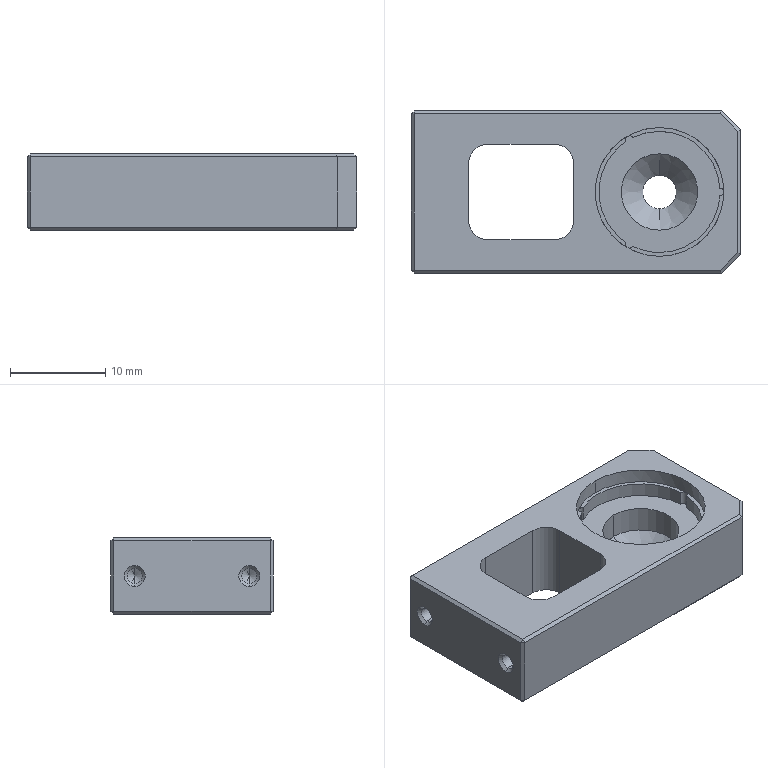CAM job | NX | 3-axis milling, drilling | part box 34.5 x 17 x 8 mm | stock box 38.5 x 21 x 9 mm
Tools:
number,name,description,diameter,corner_radius,flute_length,length,flutes
9,D10JING,Milling Tool-5 Parameters,10.0,0.0,50.0,75.0,2
7,D6A45,Milling Tool-5 Parameters,6.0,0.0,50.0,75.0,2
10,D10,Milling Tool-5 Parameters,10.0,0.0,50.0,75.0,2
8,D3R0.5,Milling Tool-5 Parameters,3.0,0.5,50.0,75.0,2
4,D4,Milling Tool-5 Parameters,4.0,0.0,50.0,75.0,2
1,D1,Milling Tool-5 Parameters,1.0,0.0,50.0,75.0,2
5,D0.5,Milling Tool-5 Parameters,0.5,0.0,50.0,75.0,2
Operations:
program,operation,operation_type,tool,method,geometry_group,spindle_rpm,surface_speed,feed_per_tooth,feed_cut,feed_plunge,cut_length_mm,path_length_mm,cut_time_min,machine_time_min
1,FLOOR_WALL,VolumeBased25DMillingOperation,D10JING,METHOD,A,9500.0,298.0,0.0658,1250.0,100.0,271.497,325.497,0.2172,0.2226
1,ZLEVEL_PROFILE,ZLevelMilling,D10,METHOD,A,9500.0,298.0,0.1316,2500.0,1000.0,2185.062,2249.863,0.8968,0.9033
1,HOLE_MILLING,CylinderMilling,D10,METHOD,A,9500.0,298.0,0.1053,2000.0,100.0,57.068,118.068,0.0285,0.0346
1,HOLE_MILLING_COPY,CylinderMilling,D10,METHOD,A,9500.0,298.0,0.1053,2000.0,100.0,43.261,107.26,0.0216,0.028
1,ZLEVEL_PROFILE_COPY_COPY,ZLevelMilling,D4,METHOD,A,9500.0,89.0,0.1053,2000.0,1000.0,411.122,476.122,0.2237,0.2302
1,ZLEVEL_PROFILE_COPY_COPY_COPY,ZLevelMilling,D4,METHOD,A,9500.0,89.0,0.1053,2000.0,1000.0,559.853,624.853,0.2981,0.3046
1,ZLEVEL_PROFILE_COPY_COPY_COPY_COPY_1,ZLevelMilling,D4,METHOD,A,9500.0,89.0,0.1053,2000.0,1000.0,130.152,195.902,0.0832,0.0898
1,ZLEVEL_PROFILE_COPY_COPY_COPY_COPY,ZLevelMilling,D4,METHOD,A,9500.0,89.0,0.0632,1200.0,1000.0,31.634,104.634,0.0268,0.0341
1,ZLEVEL_PROFILE_COPY_COPY_COPY_COPY_COPY,ZLevelMilling,D4,METHOD,A,9500.0,89.0,0.0632,1200.0,1000.0,35.227,95.227,0.0298,0.0358
1,ZLEVEL_PROFILE_COPY,ZLevelMilling,D3R0.5,METHOD,A,9500.0,89.0,0.1053,2000.0,1000.0,782.332,850.664,0.4065,0.4133
1,PLANAR_MILL_COPY_1,PlanarMilling,D6A45,METHOD,A,9500.0,179.0,0.0658,1250.0,100.0,111.117,170.117,0.0889,0.0948
1,PLANAR_MILL_COPY_1_COPY,PlanarMilling,D6A45,METHOD,A,9500.0,179.0,0.0658,1250.0,100.0,83.968,212.045,0.0672,0.08
1,DRILLING,Operation,D1,METHOD,A,4000.0,12.0,0.0088,70.0,0.0,13.5,118.133,0.1929,0.2033
1,刀补4,ZLevelMilling,D4,METHOD,A,9500.0,89.0,0.0632,1200.0,1000.0,32.268,95.268,0.0274,0.0337
1,111,ZLevelMilling,D4,METHOD,A,9500.0,298.0,0.0632,1200.0,1000.0,121.629,193.329,0.1021,0.1092
1夹着做,ZLEVEL_PROFILE_COPY_COPY_COPY_COPY_1_COPY,ZLevelMilling,D0.5,METHOD,A,9500.0,14.0,0.0421,800.0,800.0,266.785,652.354,0.3335,0.372